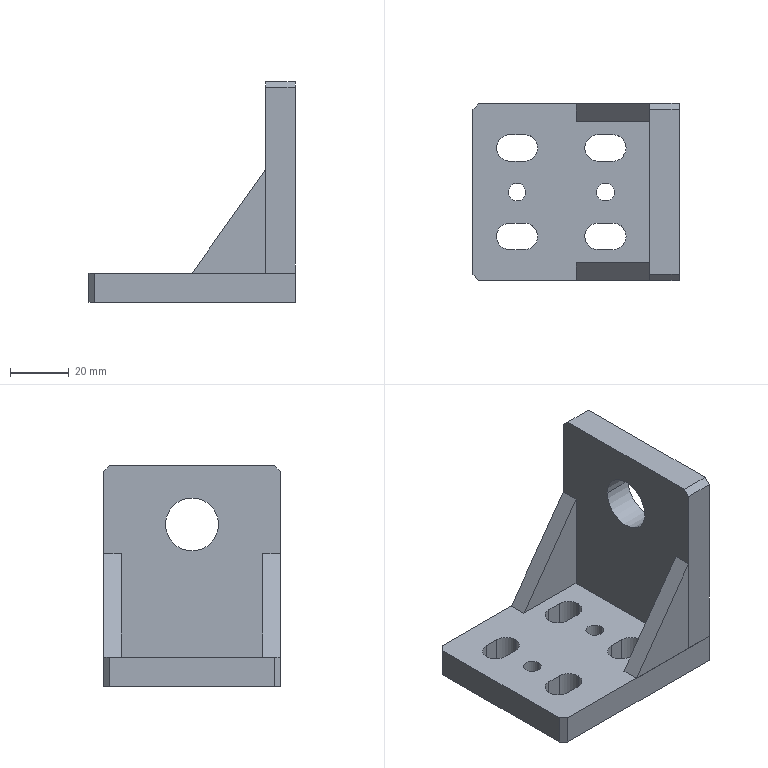Part | STEP file | Hydraulic Cylinder Connecting Bracket | 4 solids | 52 faces | box 70 x 60 x 75 mm | volume 78715 mm3 | plane 34 | cylinder 18 | commonest cylinder face diameters 9 x12 6 x4 18 x2
STEP:
#1=CARTESIAN_POINT('',(-13.,15.,0.));
#2=VERTEX_POINT('',#1);
#3=CARTESIAN_POINT('',(-17.5,19.5,0.));
#4=VERTEX_POINT('',#3);
#5=CARTESIAN_POINT('',(-17.5,15.,0.));
#6=DIRECTION('',(0.,0.,1.));
#7=DIRECTION('',(1.,0.,0.));
#8=AXIS2_PLACEMENT_3D('',#5,#6,#7);
#9=CIRCLE('',#8,4.5);
#10=EDGE_CURVE('',#2,#4,#9,.T.);
#11=ORIENTED_EDGE('',*,*,#10,.F.);
#12=CARTESIAN_POINT('',(-13.,15.,10.));
#13=VERTEX_POINT('',#12);
#14=CARTESIAN_POINT('',(-13.,15.,0.));
#15=DIRECTION('',(0.,0.,1.));
#16=VECTOR('',#15,1000.);
#17=LINE('',#14,#16);
#18=EDGE_CURVE('',#2,#13,#17,.T.);
#19=ORIENTED_EDGE('',*,*,#18,.T.);
#20=CARTESIAN_POINT('',(-17.5,19.5,10.));
#21=VERTEX_POINT('',#20);
#22=CARTESIAN_POINT('',(-17.5,15.,10.));
#23=DIRECTION('',(0.,0.,1.));
#24=DIRECTION('',(1.,0.,0.));
#25=AXIS2_PLACEMENT_3D('',#22,#23,#24);
#26=CIRCLE('',#25,4.5);
#27=EDGE_CURVE('',#13,#21,#26,.T.);
#28=ORIENTED_EDGE('',*,*,#27,.T.);
#29=CARTESIAN_POINT('',(-17.5,19.5,0.));
#30=DIRECTION('',(0.,0.,-1.));
#31=VECTOR('',#30,1000.);
#32=LINE('',#29,#31);
#33=EDGE_CURVE('',#21,#4,#32,.T.);
#34=ORIENTED_EDGE('',*,*,#33,.T.);
#35=EDGE_LOOP('',(#11,#19,#28,#34));
#36=FACE_OUTER_BOUND('',#35,.T.);
#37=CARTESIAN_POINT('',(-17.5,15.,0.));
#38=DIRECTION('',(0.,0.,1.));
#39=DIRECTION('',(1.,0.,0.));
#40=AXIS2_PLACEMENT_3D('',#37,#38,#39);
#41=CYLINDRICAL_SURFACE('',#40,4.5);
#42=ADVANCED_FACE('',(#36),#41,.F.);
#43=CARTESIAN_POINT('',(17.,15.,0.));
#44=VERTEX_POINT('',#43);
#45=CARTESIAN_POINT('',(12.5,19.5,0.));
#46=VERTEX_POINT('',#45);
#47=CARTESIAN_POINT('',(12.5,15.,0.));
#48=DIRECTION('',(0.,0.,1.));
#49=DIRECTION('',(1.,0.,0.));
#50=AXIS2_PLACEMENT_3D('',#47,#48,#49);
#51=CIRCLE('',#50,4.5);
#52=EDGE_CURVE('',#44,#46,#51,.T.);
#53=ORIENTED_EDGE('',*,*,#52,.F.);
#54=CARTESIAN_POINT('',(17.,15.,10.));
#55=VERTEX_POINT('',#54);
#56=CARTESIAN_POINT('',(17.,15.,0.));
#57=DIRECTION('',(0.,0.,1.));
#58=VECTOR('',#57,1000.);
#59=LINE('',#56,#58);
#60=EDGE_CURVE('',#44,#55,#59,.T.);
#61=ORIENTED_EDGE('',*,*,#60,.T.);
#62=CARTESIAN_POINT('',(12.5,19.5,10.));
#63=VERTEX_POINT('',#62);
#64=CARTESIAN_POINT('',(12.5,15.,10.));
#65=DIRECTION('',(0.,0.,1.));
#66=DIRECTION('',(1.,0.,0.));
#67=AXIS2_PLACEMENT_3D('',#64,#65,#66);
#68=CIRCLE('',#67,4.5);
#69=EDGE_CURVE('',#55,#63,#68,.T.);
#70=ORIENTED_EDGE('',*,*,#69,.T.);
#71=CARTESIAN_POINT('',(12.5,19.5,0.));
#72=DIRECTION('',(0.,0.,-1.));
#73=VECTOR('',#72,1000.);
#74=LINE('',#71,#73);
#75=EDGE_CURVE('',#63,#46,#74,.T.);
#76=ORIENTED_EDGE('',*,*,#75,.T.);
#77=EDGE_LOOP('',(#53,#61,#70,#76));
#78=FACE_OUTER_BOUND('',#77,.T.);
#79=CARTESIAN_POINT('',(12.5,15.,0.));
#80=DIRECTION('',(0.,0.,1.));
#81=DIRECTION('',(1.,0.,0.));
#82=AXIS2_PLACEMENT_3D('',#79,#80,#81);
#83=CYLINDRICAL_SURFACE('',#82,4.5);
#84=ADVANCED_FACE('',(#78),#83,.F.);
#85=CARTESIAN_POINT('',(17.,-15.,0.));
#86=VERTEX_POINT('',#85);
#87=CARTESIAN_POINT('',(12.5,-10.5,0.));
#88=VERTEX_POINT('',#87);
#89=CARTESIAN_POINT('',(12.5,-15.,0.));
#90=DIRECTION('',(0.,0.,1.));
#91=DIRECTION('',(1.,0.,0.));
#92=AXIS2_PLACEMENT_3D('',#89,#90,#91);
#93=CIRCLE('',#92,4.5);
#94=EDGE_CURVE('',#86,#88,#93,.T.);
#95=ORIENTED_EDGE('',*,*,#94,.F.);
#96=CARTESIAN_POINT('',(17.,-15.,10.));
#97=VERTEX_POINT('',#96);
#98=CARTESIAN_POINT('',(17.,-15.,0.));
#99=DIRECTION('',(0.,0.,1.));
#100=VECTOR('',#99,1000.);
#101=LINE('',#98,#100);
#102=EDGE_CURVE('',#86,#97,#101,.T.);
#103=ORIENTED_EDGE('',*,*,#102,.T.);
#104=CARTESIAN_POINT('',(12.5,-10.5,10.));
#105=VERTEX_POINT('',#104);
#106=CARTESIAN_POINT('',(12.5,-15.,10.));
#107=DIRECTION('',(0.,0.,1.));
#108=DIRECTION('',(1.,0.,0.));
#109=AXIS2_PLACEMENT_3D('',#106,#107,#108);
#110=CIRCLE('',#109,4.5);
#111=EDGE_CURVE('',#97,#105,#110,.T.);
#112=ORIENTED_EDGE('',*,*,#111,.T.);
#113=CARTESIAN_POINT('',(12.5,-10.5,0.));
#114=DIRECTION('',(0.,0.,-1.));
#115=VECTOR('',#114,1000.);
#116=LINE('',#113,#115);
#117=EDGE_CURVE('',#105,#88,#116,.T.);
#118=ORIENTED_EDGE('',*,*,#117,.T.);
#119=EDGE_LOOP('',(#95,#103,#112,#118));
#120=FACE_OUTER_BOUND('',#119,.T.);
#121=CARTESIAN_POINT('',(12.5,-15.,0.));
#122=DIRECTION('',(0.,0.,1.));
#123=DIRECTION('',(1.,0.,0.));
#124=AXIS2_PLACEMENT_3D('',#121,#122,#123);
#125=CYLINDRICAL_SURFACE('',#124,4.5);
#126=ADVANCED_FACE('',(#120),#125,.F.);
#127=CARTESIAN_POINT('',(-13.,-15.,0.));
#128=VERTEX_POINT('',#127);
#129=CARTESIAN_POINT('',(-17.5,-10.5,0.));
#130=VERTEX_POINT('',#129);
#131=CARTESIAN_POINT('',(-17.5,-15.,0.));
#132=DIRECTION('',(0.,0.,1.));
#133=DIRECTION('',(1.,0.,0.));
#134=AXIS2_PLACEMENT_3D('',#131,#132,#133);
#135=CIRCLE('',#134,4.5);
#136=EDGE_CURVE('',#128,#130,#135,.T.);
#137=ORIENTED_EDGE('',*,*,#136,.F.);
#138=CARTESIAN_POINT('',(-13.,-15.,10.));
#139=VERTEX_POINT('',#138);
#140=CARTESIAN_POINT('',(-13.,-15.,0.));
#141=DIRECTION('',(0.,0.,1.));
#142=VECTOR('',#141,1000.);
#143=LINE('',#140,#142);
#144=EDGE_CURVE('',#128,#139,#143,.T.);
#145=ORIENTED_EDGE('',*,*,#144,.T.);
#146=CARTESIAN_POINT('',(-17.5,-10.5,10.));
#147=VERTEX_POINT('',#146);
#148=CARTESIAN_POINT('',(-17.5,-15.,10.));
#149=DIRECTION('',(0.,0.,1.));
#150=DIRECTION('',(1.,0.,0.));
#151=AXIS2_PLACEMENT_3D('',#148,#149,#150);
#152=CIRCLE('',#151,4.5);
#153=EDGE_CURVE('',#139,#147,#152,.T.);
#154=ORIENTED_EDGE('',*,*,#153,.T.);
#155=CARTESIAN_POINT('',(-17.5,-10.5,0.));
#156=DIRECTION('',(0.,0.,-1.));
#157=VECTOR('',#156,1000.);
#158=LINE('',#155,#157);
#159=EDGE_CURVE('',#147,#130,#158,.T.);
#160=ORIENTED_EDGE('',*,*,#159,.T.);
#161=EDGE_LOOP('',(#137,#145,#154,#160));
#162=FACE_OUTER_BOUND('',#161,.T.);
#163=CARTESIAN_POINT('',(-17.5,-15.,0.));
#164=DIRECTION('',(0.,0.,1.));
#165=DIRECTION('',(1.,0.,0.));
#166=AXIS2_PLACEMENT_3D('',#163,#164,#165);
#167=CYLINDRICAL_SURFACE('',#166,4.5);
#168=ADVANCED_FACE('',(#162),#167,.F.);
#169=CARTESIAN_POINT('',(-23.,0.,0.));
#170=VERTEX_POINT('',#169);
#171=CARTESIAN_POINT('',(-17.,0.,0.));
#172=VERTEX_POINT('',#171);
#173=CARTESIAN_POINT('',(-20.,0.,0.));
#174=DIRECTION('',(0.,0.,1.));
#175=DIRECTION('',(1.,0.,0.));
#176=AXIS2_PLACEMENT_3D('',#173,#174,#175);
#177=CIRCLE('',#176,3.);
#178=EDGE_CURVE('',#170,#172,#177,.T.);
#179=ORIENTED_EDGE('',*,*,#178,.F.);
#180=CARTESIAN_POINT('',(-23.,0.,10.));
#181=VERTEX_POINT('',#180);
#182=CARTESIAN_POINT('',(-23.,0.,0.));
#183=DIRECTION('',(0.,0.,1.));
#184=VECTOR('',#183,1000.);
#185=LINE('',#182,#184);
#186=EDGE_CURVE('',#170,#181,#185,.T.);
#187=ORIENTED_EDGE('',*,*,#186,.T.);
#188=CARTESIAN_POINT('',(-17.,0.,10.));
#189=VERTEX_POINT('',#188);
#190=CARTESIAN_POINT('',(-20.,0.,10.));
#191=DIRECTION('',(0.,0.,1.));
#192=DIRECTION('',(1.,0.,0.));
#193=AXIS2_PLACEMENT_3D('',#190,#191,#192);
#194=CIRCLE('',#193,3.);
#195=EDGE_CURVE('',#181,#189,#194,.T.);
#196=ORIENTED_EDGE('',*,*,#195,.T.);
#197=CARTESIAN_POINT('',(-17.,0.,0.));
#198=DIRECTION('',(0.,0.,1.));
#199=VECTOR('',#198,1000.);
#200=LINE('',#197,#199);
#201=EDGE_CURVE('',#172,#189,#200,.T.);
#202=ORIENTED_EDGE('',*,*,#201,.F.);
#203=EDGE_LOOP('',(#179,#187,#196,#202));
#204=FACE_OUTER_BOUND('',#203,.T.);
#205=CARTESIAN_POINT('',(-20.,0.,0.));
#206=DIRECTION('',(0.,0.,1.));
#207=DIRECTION('',(1.,0.,0.));
#208=AXIS2_PLACEMENT_3D('',#205,#206,#207);
#209=CYLINDRICAL_SURFACE('',#208,3.);
#210=ADVANCED_FACE('',(#204),#209,.F.);
#211=CARTESIAN_POINT('',(7.,0.,0.));
#212=VERTEX_POINT('',#211);
#213=CARTESIAN_POINT('',(13.,0.,0.));
#214=VERTEX_POINT('',#213);
#215=CARTESIAN_POINT('',(10.,0.,0.));
#216=DIRECTION('',(0.,0.,1.));
#217=DIRECTION('',(1.,0.,0.));
#218=AXIS2_PLACEMENT_3D('',#215,#216,#217);
#219=CIRCLE('',#218,3.);
#220=EDGE_CURVE('',#212,#214,#219,.T.);
#221=ORIENTED_EDGE('',*,*,#220,.F.);
#222=CARTESIAN_POINT('',(7.,0.,10.));
#223=VERTEX_POINT('',#222);
#224=CARTESIAN_POINT('',(7.,0.,0.));
#225=DIRECTION('',(0.,0.,1.));
#226=VECTOR('',#225,1000.);
#227=LINE('',#224,#226);
#228=EDGE_CURVE('',#212,#223,#227,.T.);
#229=ORIENTED_EDGE('',*,*,#228,.T.);
#230=CARTESIAN_POINT('',(13.,0.,10.));
#231=VERTEX_POINT('',#230);
#232=CARTESIAN_POINT('',(10.,0.,10.));
#233=DIRECTION('',(0.,0.,1.));
#234=DIRECTION('',(1.,0.,0.));
#235=AXIS2_PLACEMENT_3D('',#232,#233,#234);
#236=CIRCLE('',#235,3.);
#237=EDGE_CURVE('',#223,#231,#236,.T.);
#238=ORIENTED_EDGE('',*,*,#237,.T.);
#239=CARTESIAN_POINT('',(13.,0.,0.));
#240=DIRECTION('',(0.,0.,1.));
#241=VECTOR('',#240,1000.);
#242=LINE('',#239,#241);
#243=EDGE_CURVE('',#214,#231,#242,.T.);
#244=ORIENTED_EDGE('',*,*,#243,.F.);
#245=EDGE_LOOP('',(#221,#229,#238,#244));
#246=FACE_OUTER_BOUND('',#245,.T.);
#247=CARTESIAN_POINT('',(10.,0.,0.));
#248=DIRECTION('',(0.,0.,1.));
#249=DIRECTION('',(1.,0.,0.));
#250=AXIS2_PLACEMENT_3D('',#247,#248,#249);
#251=CYLINDRICAL_SURFACE('',#250,3.);
#252=ADVANCED_FACE('',(#246),#251,.F.);
#253=CARTESIAN_POINT('',(-33.,-30.,10.));
#254=VERTEX_POINT('',#253);
#255=CARTESIAN_POINT('',(-35.,-28.,10.));
#256=VERTEX_POINT('',#255);
#257=CARTESIAN_POINT('',(-33.,-30.,10.));
#258=DIRECTION('',(-0.7071,0.7071,0.));
#259=VECTOR('',#258,1000.);
#260=LINE('',#257,#259);
#261=EDGE_CURVE('',#254,#256,#260,.T.);
#262=ORIENTED_EDGE('',*,*,#261,.F.);
#263=CARTESIAN_POINT('',(35.,-30.,10.));
#264=VERTEX_POINT('',#263);
#265=CARTESIAN_POINT('',(0.,-30.,10.));
#266=DIRECTION('',(-1.,0.,0.));
#267=VECTOR('',#266,1000.);
#268=LINE('',#265,#267);
#269=EDGE_CURVE('',#264,#254,#268,.T.);
#270=ORIENTED_EDGE('',*,*,#269,.F.);
#271=CARTESIAN_POINT('',(35.,30.,10.));
#272=VERTEX_POINT('',#271);
#273=CARTESIAN_POINT('',(35.,0.,10.));
#274=DIRECTION('',(0.,-1.,0.));
#275=VECTOR('',#274,1000.);
#276=LINE('',#273,#275);
#277=EDGE_CURVE('',#272,#264,#276,.T.);
#278=ORIENTED_EDGE('',*,*,#277,.F.);
#279=CARTESIAN_POINT('',(-33.,30.,10.));
#280=VERTEX_POINT('',#279);
#281=CARTESIAN_POINT('',(0.,30.,10.));
#282=DIRECTION('',(1.,0.,0.));
#283=VECTOR('',#282,1000.);
#284=LINE('',#281,#283);
#285=EDGE_CURVE('',#280,#272,#284,.T.);
#286=ORIENTED_EDGE('',*,*,#285,.F.);
#287=CARTESIAN_POINT('',(-35.,28.,10.));
#288=VERTEX_POINT('',#287);
#289=CARTESIAN_POINT('',(-35.,28.,10.));
#290=DIRECTION('',(0.7071,0.7071,0.));
#291=VECTOR('',#290,1000.);
#292=LINE('',#289,#291);
#293=EDGE_CURVE('',#288,#280,#292,.T.);
#294=ORIENTED_EDGE('',*,*,#293,.F.);
#295=CARTESIAN_POINT('',(-35.,0.,10.));
#296=DIRECTION('',(0.,1.,0.));
#297=VECTOR('',#296,1000.);
#298=LINE('',#295,#297);
#299=EDGE_CURVE('',#256,#288,#298,.T.);
#300=ORIENTED_EDGE('',*,*,#299,.F.);
#301=EDGE_LOOP('',(#262,#270,#278,#286,#294,#300));
#302=FACE_OUTER_BOUND('',#301,.T.);
#303=CARTESIAN_POINT('',(-22.5,19.5,10.));
#304=VERTEX_POINT('',#303);
#305=CARTESIAN_POINT('',(-22.5,10.5,10.));
#306=VERTEX_POINT('',#305);
#307=CARTESIAN_POINT('',(-22.5,15.,10.));
#308=DIRECTION('',(0.,0.,1.));
#309=DIRECTION('',(1.,0.,0.));
#310=AXIS2_PLACEMENT_3D('',#307,#308,#309);
#311=CIRCLE('',#310,4.5);
#312=EDGE_CURVE('',#304,#306,#311,.T.);
#313=ORIENTED_EDGE('',*,*,#312,.F.);
#314=CARTESIAN_POINT('',(0.,19.5,10.));
#315=DIRECTION('',(-1.,0.,0.));
#316=VECTOR('',#315,1000.);
#317=LINE('',#314,#316);
#318=EDGE_CURVE('',#21,#304,#317,.T.);
#319=ORIENTED_EDGE('',*,*,#318,.F.);
#320=ORIENTED_EDGE('',*,*,#27,.F.);
#321=CARTESIAN_POINT('',(-17.5,10.5,10.));
#322=VERTEX_POINT('',#321);
#323=CARTESIAN_POINT('',(-17.5,15.,10.));
#324=DIRECTION('',(0.,0.,1.));
#325=DIRECTION('',(1.,0.,0.));
#326=AXIS2_PLACEMENT_3D('',#323,#324,#325);
#327=CIRCLE('',#326,4.5);
#328=EDGE_CURVE('',#322,#13,#327,.T.);
#329=ORIENTED_EDGE('',*,*,#328,.F.);
#330=CARTESIAN_POINT('',(0.,10.5,10.));
#331=DIRECTION('',(1.,0.,0.));
#332=VECTOR('',#331,1000.);
#333=LINE('',#330,#332);
#334=EDGE_CURVE('',#306,#322,#333,.T.);
#335=ORIENTED_EDGE('',*,*,#334,.F.);
#336=EDGE_LOOP('',(#313,#319,#320,#329,#335));
#337=FACE_BOUND('',#336,.T.);
#338=CARTESIAN_POINT('',(7.5,19.5,10.));
#339=VERTEX_POINT('',#338);
#340=CARTESIAN_POINT('',(7.5,10.5,10.));
#341=VERTEX_POINT('',#340);
#342=CARTESIAN_POINT('',(7.5,15.,10.));
#343=DIRECTION('',(0.,0.,1.));
#344=DIRECTION('',(1.,0.,0.));
#345=AXIS2_PLACEMENT_3D('',#342,#343,#344);
#346=CIRCLE('',#345,4.5);
#347=EDGE_CURVE('',#339,#341,#346,.T.);
#348=ORIENTED_EDGE('',*,*,#347,.F.);
#349=CARTESIAN_POINT('',(0.,19.5,10.));
#350=DIRECTION('',(-1.,0.,0.));
#351=VECTOR('',#350,1000.);
#352=LINE('',#349,#351);
#353=EDGE_CURVE('',#63,#339,#352,.T.);
#354=ORIENTED_EDGE('',*,*,#353,.F.);
#355=ORIENTED_EDGE('',*,*,#69,.F.);
#356=CARTESIAN_POINT('',(12.5,10.5,10.));
#357=VERTEX_POINT('',#356);
#358=CARTESIAN_POINT('',(12.5,15.,10.));
#359=DIRECTION('',(0.,0.,1.));
#360=DIRECTION('',(1.,0.,0.));
#361=AXIS2_PLACEMENT_3D('',#358,#359,#360);
#362=CIRCLE('',#361,4.5);
#363=EDGE_CURVE('',#357,#55,#362,.T.);
#364=ORIENTED_EDGE('',*,*,#363,.F.);
#365=CARTESIAN_POINT('',(0.,10.5,10.));
#366=DIRECTION('',(1.,0.,0.));
#367=VECTOR('',#366,1000.);
#368=LINE('',#365,#367);
#369=EDGE_CURVE('',#341,#357,#368,.T.);
#370=ORIENTED_EDGE('',*,*,#369,.F.);
#371=EDGE_LOOP('',(#348,#354,#355,#364,#370));
#372=FACE_BOUND('',#371,.T.);
#373=CARTESIAN_POINT('',(7.5,-10.5,10.));
#374=VERTEX_POINT('',#373);
#375=CARTESIAN_POINT('',(7.5,-19.5,10.));
#376=VERTEX_POINT('',#375);
#377=CARTESIAN_POINT('',(7.5,-15.,10.));
#378=DIRECTION('',(0.,0.,1.));
#379=DIRECTION('',(1.,0.,0.));
#380=AXIS2_PLACEMENT_3D('',#377,#378,#379);
#381=CIRCLE('',#380,4.5);
#382=EDGE_CURVE('',#374,#376,#381,.T.);
#383=ORIENTED_EDGE('',*,*,#382,.F.);
#384=CARTESIAN_POINT('',(0.,-10.5,10.));
#385=DIRECTION('',(-1.,0.,0.));
#386=VECTOR('',#385,1000.);
#387=LINE('',#384,#386);
#388=EDGE_CURVE('',#105,#374,#387,.T.);
#389=ORIENTED_EDGE('',*,*,#388,.F.);
#390=ORIENTED_EDGE('',*,*,#111,.F.);
#391=CARTESIAN_POINT('',(12.5,-19.5,10.));
#392=VERTEX_POINT('',#391);
#393=CARTESIAN_POINT('',(12.5,-15.,10.));
#394=DIRECTION('',(0.,0.,1.));
#395=DIRECTION('',(1.,0.,0.));
#396=AXIS2_PLACEMENT_3D('',#393,#394,#395);
#397=CIRCLE('',#396,4.5);
#398=EDGE_CURVE('',#392,#97,#397,.T.);
#399=ORIENTED_EDGE('',*,*,#398,.F.);
#400=CARTESIAN_POINT('',(0.,-19.5,10.));
#401=DIRECTION('',(1.,0.,0.));
#402=VECTOR('',#401,1000.);
#403=LINE('',#400,#402);
#404=EDGE_CURVE('',#376,#392,#403,.T.);
#405=ORIENTED_EDGE('',*,*,#404,.F.);
#406=EDGE_LOOP('',(#383,#389,#390,#399,#405));
#407=FACE_BOUND('',#406,.T.);
#408=CARTESIAN_POINT('',(-22.5,-10.5,10.));
#409=VERTEX_POINT('',#408);
#410=CARTESIAN_POINT('',(-22.5,-19.5,10.));
#411=VERTEX_POINT('',#410);
#412=CARTESIAN_POINT('',(-22.5,-15.,10.));
#413=DIRECTION('',(0.,0.,1.));
#414=DIRECTION('',(1.,0.,0.));
#415=AXIS2_PLACEMENT_3D('',#412,#413,#414);
#416=CIRCLE('',#415,4.5);
#417=EDGE_CURVE('',#409,#411,#416,.T.);
#418=ORIENTED_EDGE('',*,*,#417,.F.);
#419=CARTESIAN_POINT('',(0.,-10.5,10.));
#420=DIRECTION('',(-1.,0.,0.));
#421=VECTOR('',#420,1000.);
#422=LINE('',#419,#421);
#423=EDGE_CURVE('',#147,#409,#422,.T.);
#424=ORIENTED_EDGE('',*,*,#423,.F.);
#425=ORIENTED_EDGE('',*,*,#153,.F.);
#426=CARTESIAN_POINT('',(-17.5,-19.5,10.));
#427=VERTEX_POINT('',#426);
#428=CARTESIAN_POINT('',(-17.5,-15.,10.));
#429=DIRECTION('',(0.,0.,1.));
#430=DIRECTION('',(1.,0.,0.));
#431=AXIS2_PLACEMENT_3D('',#428,#429,#430);
#432=CIRCLE('',#431,4.5);
#433=EDGE_CURVE('',#427,#139,#432,.T.);
#434=ORIENTED_EDGE('',*,*,#433,.F.);
#435=CARTESIAN_POINT('',(0.,-19.5,10.));
#436=DIRECTION('',(1.,0.,0.));
#437=VECTOR('',#436,1000.);
#438=LINE('',#435,#437);
#439=EDGE_CURVE('',#411,#427,#438,.T.);
#440=ORIENTED_EDGE('',*,*,#439,.F.);
#441=EDGE_LOOP('',(#418,#424,#425,#434,#440));
#442=FACE_BOUND('',#441,.T.);
#443=CARTESIAN_POINT('',(-20.,0.,10.));
#444=DIRECTION('',(0.,0.,1.));
#445=DIRECTION('',(1.,0.,0.));
#446=AXIS2_PLACEMENT_3D('',#443,#444,#445);
#447=CIRCLE('',#446,3.);
#448=EDGE_CURVE('',#189,#181,#447,.T.);
#449=ORIENTED_EDGE('',*,*,#448,.F.);
#450=ORIENTED_EDGE('',*,*,#195,.F.);
#451=EDGE_LOOP('',(#449,#450));
#452=FACE_BOUND('',#451,.T.);
#453=CARTESIAN_POINT('',(10.,0.,10.));
#454=DIRECTION('',(0.,0.,1.));
#455=DIRECTION('',(1.,0.,0.));
#456=AXIS2_PLACEMENT_3D('',#453,#454,#455);
#457=CIRCLE('',#456,3.);
#458=EDGE_CURVE('',#231,#223,#457,.T.);
#459=ORIENTED_EDGE('',*,*,#458,.F.);
#460=ORIENTED_EDGE('',*,*,#237,.F.);
#461=EDGE_LOOP('',(#459,#460));
#462=FACE_BOUND('',#461,.T.);
#463=CARTESIAN_POINT('',(0.,0.,10.));
#464=DIRECTION('',(0.,0.,-1.));
#465=DIRECTION('',(-1.,0.,0.));
#466=AXIS2_PLACEMENT_3D('',#463,#464,#465);
#467=PLANE('',#466);
#468=ADVANCED_FACE('',(#302,#337,#372,#407,#442,#452,#462),#467,.F.);
#469=ORIENTED_EDGE('',*,*,#299,.T.);
#470=CARTESIAN_POINT('',(-35.,28.,0.));
#471=VERTEX_POINT('',#470);
#472=CARTESIAN_POINT('',(-35.,28.,10.));
#473=DIRECTION('',(0.,0.,-1.));
#474=VECTOR('',#473,1000.);
#475=LINE('',#472,#474);
#476=EDGE_CURVE('',#288,#471,#475,.T.);
#477=ORIENTED_EDGE('',*,*,#476,.T.);
#478=CARTESIAN_POINT('',(-35.,-28.,0.));
#479=VERTEX_POINT('',#478);
#480=CARTESIAN_POINT('',(-35.,-30.,0.));
#481=DIRECTION('',(0.,-1.,0.));
#482=VECTOR('',#481,1000.);
#483=LINE('',#480,#482);
#484=EDGE_CURVE('',#471,#479,#483,.T.);
#485=ORIENTED_EDGE('',*,*,#484,.T.);
#486=CARTESIAN_POINT('',(-35.,-28.,10.));
#487=DIRECTION('',(0.,0.,1.));
#488=VECTOR('',#487,1000.);
#489=LINE('',#486,#488);
#490=EDGE_CURVE('',#479,#256,#489,.T.);
#491=ORIENTED_EDGE('',*,*,#490,.T.);
#492=EDGE_LOOP('',(#469,#477,#485,#491));
#493=FACE_OUTER_BOUND('',#492,.T.);
#494=CARTESIAN_POINT('',(-35.,-30.,10.));
#495=DIRECTION('',(-1.,0.,0.));
#496=DIRECTION('',(0.,0.,1.));
#497=AXIS2_PLACEMENT_3D('',#494,#495,#496);
#498=PLANE('',#497);
#499=ADVANCED_FACE('',(#493),#498,.T.);
#500=CARTESIAN_POINT('',(-33.,-30.,0.));
#501=VERTEX_POINT('',#500);
#502=CARTESIAN_POINT('',(-33.,-30.,0.));
#503=DIRECTION('',(0.7071,-0.7071,0.));
#504=VECTOR('',#503,1000.);
#505=LINE('',#502,#504);
#506=EDGE_CURVE('',#479,#501,#505,.T.);
#507=ORIENTED_EDGE('',*,*,#506,.T.);
#508=CARTESIAN_POINT('',(-33.,-30.,10.));
#509=DIRECTION('',(0.,0.,1.));
#510=VECTOR('',#509,1000.);
#511=LINE('',#508,#510);
#512=EDGE_CURVE('',#501,#254,#511,.T.);
#513=ORIENTED_EDGE('',*,*,#512,.T.);
#514=ORIENTED_EDGE('',*,*,#261,.T.);
#515=ORIENTED_EDGE('',*,*,#490,.F.);
#516=EDGE_LOOP('',(#507,#513,#514,#515));
#517=FACE_OUTER_BOUND('',#516,.T.);
#518=CARTESIAN_POINT('',(-33.,-30.,10.));
#519=DIRECTION('',(-0.7071,-0.7071,0.));
#520=DIRECTION('',(0.7071,-0.7071,0.));
#521=AXIS2_PLACEMENT_3D('',#518,#519,#520);
#522=PLANE('',#521);
#523=ADVANCED_FACE('',(#517),#522,.T.);
#524=ORIENTED_EDGE('',*,*,#512,.F.);
#525=CARTESIAN_POINT('',(35.,-30.,0.));
#526=VERTEX_POINT('',#525);
#527=CARTESIAN_POINT('',(-35.,-30.,0.));
#528=DIRECTION('',(-1.,0.,0.));
#529=VECTOR('',#528,1000.);
#530=LINE('',#527,#529);
#531=EDGE_CURVE('',#526,#501,#530,.T.);
#532=ORIENTED_EDGE('',*,*,#531,.F.);
#533=CARTESIAN_POINT('',(35.,-30.,10.));
#534=DIRECTION('',(0.,0.,-1.));
#535=VECTOR('',#534,1000.);
#536=LINE('',#533,#535);
#537=EDGE_CURVE('',#264,#526,#536,.T.);
#538=ORIENTED_EDGE('',*,*,#537,.F.);
#539=ORIENTED_EDGE('',*,*,#269,.T.);
#540=EDGE_LOOP('',(#524,#532,#538,#539));
#541=FACE_OUTER_BOUND('',#540,.T.);
#542=CARTESIAN_POINT('',(-35.,-30.,10.));
#543=DIRECTION('',(0.,1.,0.));
#544=DIRECTION('',(-1.,0.,0.));
#545=AXIS2_PLACEMENT_3D('',#542,#543,#544);
#546=PLANE('',#545);
#547=ADVANCED_FACE('',(#541),#546,.F.);
#548=ORIENTED_EDGE('',*,*,#277,.T.);
#549=ORIENTED_EDGE('',*,*,#537,.T.);
#550=CARTESIAN_POINT('',(35.,30.,0.));
#551=VERTEX_POINT('',#550);
#552=CARTESIAN_POINT('',(35.,30.,0.));
#553=DIRECTION('',(0.,1.,0.));
#554=VECTOR('',#553,1000.);
#555=LINE('',#552,#554);
#556=EDGE_CURVE('',#526,#551,#555,.T.);
#557=ORIENTED_EDGE('',*,*,#556,.T.);
#558=CARTESIAN_POINT('',(35.,30.,10.));
#559=DIRECTION('',(0.,0.,1.));
#560=VECTOR('',#559,1000.);
#561=LINE('',#558,#560);
#562=EDGE_CURVE('',#551,#272,#561,.T.);
#563=ORIENTED_EDGE('',*,*,#562,.T.);
#564=EDGE_LOOP('',(#548,#549,#557,#563));
#565=FACE_OUTER_BOUND('',#564,.T.);
#566=CARTESIAN_POINT('',(35.,30.,10.));
#567=DIRECTION('',(1.,0.,0.));
#568=DIRECTION('',(0.,0.,-1.));
#569=AXIS2_PLACEMENT_3D('',#566,#567,#568);
#570=PLANE('',#569);
#571=ADVANCED_FACE('',(#565),#570,.T.);
#572=ORIENTED_EDGE('',*,*,#285,.T.);
#573=ORIENTED_EDGE('',*,*,#562,.F.);
#574=CARTESIAN_POINT('',(-33.,30.,0.));
#575=VERTEX_POINT('',#574);
#576=CARTESIAN_POINT('',(-35.,30.,0.));
#577=DIRECTION('',(-1.,0.,0.));
#578=VECTOR('',#577,1000.);
#579=LINE('',#576,#578);
#580=EDGE_CURVE('',#551,#575,#579,.T.);
#581=ORIENTED_EDGE('',*,*,#580,.T.);
#582=CARTESIAN_POINT('',(-33.,30.,10.));
#583=DIRECTION('',(0.,0.,1.));
#584=VECTOR('',#583,1000.);
#585=LINE('',#582,#584);
#586=EDGE_CURVE('',#575,#280,#585,.T.);
#587=ORIENTED_EDGE('',*,*,#586,.T.);
#588=EDGE_LOOP('',(#572,#573,#581,#587));
#589=FACE_OUTER_BOUND('',#588,.T.);
#590=CARTESIAN_POINT('',(-35.,30.,10.));
#591=DIRECTION('',(0.,1.,0.));
#592=DIRECTION('',(-1.,0.,0.));
#593=AXIS2_PLACEMENT_3D('',#590,#591,#592);
#594=PLANE('',#593);
#595=ADVANCED_FACE('',(#589),#594,.T.);
#596=ORIENTED_EDGE('',*,*,#586,.F.);
#597=CARTESIAN_POINT('',(-35.,28.,0.));
#598=DIRECTION('',(0.7071,0.7071,0.));
#599=VECTOR('',#598,1000.);
#600=LINE('',#597,#599);
#601=EDGE_CURVE('',#471,#575,#600,.T.);
#602=ORIENTED_EDGE('',*,*,#601,.F.);
#603=ORIENTED_EDGE('',*,*,#476,.F.);
#604=ORIENTED_EDGE('',*,*,#293,.T.);
#605=EDGE_LOOP('',(#596,#602,#603,#604));
#606=FACE_OUTER_BOUND('',#605,.T.);
#607=CARTESIAN_POINT('',(-35.,28.,10.));
#608=DIRECTION('',(0.7071,-0.7071,0.));
#609=DIRECTION('',(0.7071,0.7071,0.));
#610=AXIS2_PLACEMENT_3D('',#607,#608,#609);
#611=PLANE('',#610);
#612=ADVANCED_FACE('',(#606),#611,.F.);
#613=CARTESIAN_POINT('',(-17.5,10.5,0.));
#614=VERTEX_POINT('',#613);
#615=CARTESIAN_POINT('',(-17.5,10.5,0.));
#616=DIRECTION('',(0.,0.,1.));
#617=VECTOR('',#616,1000.);
#618=LINE('',#615,#617);
#619=EDGE_CURVE('',#614,#322,#618,.T.);
#620=ORIENTED_EDGE('',*,*,#619,.F.);
#621=CARTESIAN_POINT('',(-22.5,10.5,0.));
#622=VERTEX_POINT('',#621);
#623=CARTESIAN_POINT('',(-22.5,10.5,0.));
#624=DIRECTION('',(1.,0.,0.));
#625=VECTOR('',#624,1000.);
#626=LINE('',#623,#625);
#627=EDGE_CURVE('',#622,#614,#626,.T.);
#628=ORIENTED_EDGE('',*,*,#627,.F.);
#629=CARTESIAN_POINT('',(-22.5,10.5,0.));
#630=DIRECTION('',(0.,0.,-1.));
#631=VECTOR('',#630,1000.);
#632=LINE('',#629,#631);
#633=EDGE_CURVE('',#306,#622,#632,.T.);
#634=ORIENTED_EDGE('',*,*,#633,.F.);
#635=ORIENTED_EDGE('',*,*,#334,.T.);
#636=EDGE_LOOP('',(#620,#628,#634,#635));
#637=FACE_OUTER_BOUND('',#636,.T.);
#638=CARTESIAN_POINT('',(-22.5,10.5,0.));
#639=DIRECTION('',(0.,-1.,0.));
#640=DIRECTION('',(1.,0.,0.));
#641=AXIS2_PLACEMENT_3D('',#638,#639,#640);
#642=PLANE('',#641);
#643=ADVANCED_FACE('',(#637),#642,.F.);
#644=ORIENTED_EDGE('',*,*,#633,.T.);
#645=CARTESIAN_POINT('',(-22.5,19.5,0.));
#646=VERTEX_POINT('',#645);
#647=CARTESIAN_POINT('',(-22.5,15.,0.));
#648=DIRECTION('',(0.,0.,1.));
#649=DIRECTION('',(1.,0.,0.));
#650=AXIS2_PLACEMENT_3D('',#647,#648,#649);
#651=CIRCLE('',#650,4.5);
#652=EDGE_CURVE('',#646,#622,#651,.T.);
#653=ORIENTED_EDGE('',*,*,#652,.F.);
#654=CARTESIAN_POINT('',(-22.5,19.5,0.));
#655=DIRECTION('',(0.,0.,-1.));
#656=VECTOR('',#655,1000.);
#657=LINE('',#654,#656);
#658=EDGE_CURVE('',#304,#646,#657,.T.);
#659=ORIENTED_EDGE('',*,*,#658,.F.);
#660=ORIENTED_EDGE('',*,*,#312,.T.);
#661=EDGE_LOOP('',(#644,#653,#659,#660));
#662=FACE_OUTER_BOUND('',#661,.T.);
#663=CARTESIAN_POINT('',(-22.5,15.,0.));
#664=DIRECTION('',(0.,0.,1.));
#665=DIRECTION('',(1.,0.,0.));
#666=AXIS2_PLACEMENT_3D('',#663,#664,#665);
#667=CYLINDRICAL_SURFACE('',#666,4.5);
#668=ADVANCED_FACE('',(#662),#667,.F.);
#669=ORIENTED_EDGE('',*,*,#658,.T.);
#670=CARTESIAN_POINT('',(-22.5,19.5,0.));
#671=DIRECTION('',(-1.,0.,0.));
#672=VECTOR('',#671,1000.);
#673=LINE('',#670,#672);
#674=EDGE_CURVE('',#4,#646,#673,.T.);
#675=ORIENTED_EDGE('',*,*,#674,.F.);
#676=ORIENTED_EDGE('',*,*,#33,.F.);
#677=ORIENTED_EDGE('',*,*,#318,.T.);
#678=EDGE_LOOP('',(#669,#675,#676,#677));
#679=FACE_OUTER_BOUND('',#678,.T.);
#680=CARTESIAN_POINT('',(-22.5,19.5,0.));
#681=DIRECTION('',(0.,1.,0.));
#682=DIRECTION('',(0.,0.,1.));
#683=AXIS2_PLACEMENT_3D('',#680,#681,#682);
#684=PLANE('',#683);
#685=ADVANCED_FACE('',(#679),#684,.F.);
#686=ORIENTED_EDGE('',*,*,#18,.F.);
#687=CARTESIAN_POINT('',(-17.5,15.,0.));
#688=DIRECTION('',(0.,0.,1.));
#689=DIRECTION('',(1.,0.,0.));
#690=AXIS2_PLACEMENT_3D('',#687,#688,#689);
#691=CIRCLE('',#690,4.5);
#692=EDGE_CURVE('',#614,#2,#691,.T.);
#693=ORIENTED_EDGE('',*,*,#692,.F.);
#694=ORIENTED_EDGE('',*,*,#619,.T.);
#695=ORIENTED_EDGE('',*,*,#328,.T.);
#696=EDGE_LOOP('',(#686,#693,#694,#695));
#697=FACE_OUTER_BOUND('',#696,.T.);
#698=CARTESIAN_POINT('',(-17.5,15.,0.));
#699=DIRECTION('',(0.,0.,1.));
#700=DIRECTION('',(1.,0.,0.));
#701=AXIS2_PLACEMENT_3D('',#698,#699,#700);
#702=CYLINDRICAL_SURFACE('',#701,4.5);
#703=ADVANCED_FACE('',(#697),#702,.F.);
#704=CARTESIAN_POINT('',(12.5,10.5,0.));
#705=VERTEX_POINT('',#704);
#706=CARTESIAN_POINT('',(12.5,10.5,0.));
#707=DIRECTION('',(0.,0.,1.));
#708=VECTOR('',#707,1000.);
#709=LINE('',#706,#708);
#710=EDGE_CURVE('',#705,#357,#709,.T.);
#711=ORIENTED_EDGE('',*,*,#710,.F.);
#712=CARTESIAN_POINT('',(7.5,10.5,0.));
#713=VERTEX_POINT('',#712);
#714=CARTESIAN_POINT('',(7.5,10.5,0.));
#715=DIRECTION('',(1.,0.,0.));
#716=VECTOR('',#715,1000.);
#717=LINE('',#714,#716);
#718=EDGE_CURVE('',#713,#705,#717,.T.);
#719=ORIENTED_EDGE('',*,*,#718,.F.);
#720=CARTESIAN_POINT('',(7.5,10.5,0.));
#721=DIRECTION('',(0.,0.,-1.));
#722=VECTOR('',#721,1000.);
#723=LINE('',#720,#722);
#724=EDGE_CURVE('',#341,#713,#723,.T.);
#725=ORIENTED_EDGE('',*,*,#724,.F.);
#726=ORIENTED_EDGE('',*,*,#369,.T.);
#727=EDGE_LOOP('',(#711,#719,#725,#726));
#728=FACE_OUTER_BOUND('',#727,.T.);
#729=CARTESIAN_POINT('',(7.5,10.5,0.));
#730=DIRECTION('',(0.,-1.,0.));
#731=DIRECTION('',(1.,0.,0.));
#732=AXIS2_PLACEMENT_3D('',#729,#730,#731);
#733=PLANE('',#732);
#734=ADVANCED_FACE('',(#728),#733,.F.);
#735=ORIENTED_EDGE('',*,*,#724,.T.);
#736=CARTESIAN_POINT('',(7.5,19.5,0.));
#737=VERTEX_POINT('',#736);
#738=CARTESIAN_POINT('',(7.5,15.,0.));
#739=DIRECTION('',(0.,0.,1.));
#740=DIRECTION('',(1.,0.,0.));
#741=AXIS2_PLACEMENT_3D('',#738,#739,#740);
#742=CIRCLE('',#741,4.5);
#743=EDGE_CURVE('',#737,#713,#742,.T.);
#744=ORIENTED_EDGE('',*,*,#743,.F.);
#745=CARTESIAN_POINT('',(7.5,19.5,0.));
#746=DIRECTION('',(0.,0.,-1.));
#747=VECTOR('',#746,1000.);
#748=LINE('',#745,#747);
#749=EDGE_CURVE('',#339,#737,#748,.T.);
#750=ORIENTED_EDGE('',*,*,#749,.F.);
#751=ORIENTED_EDGE('',*,*,#347,.T.);
#752=EDGE_LOOP('',(#735,#744,#750,#751));
#753=FACE_OUTER_BOUND('',#752,.T.);
#754=CARTESIAN_POINT('',(7.5,15.,0.));
#755=DIRECTION('',(0.,0.,1.));
#756=DIRECTION('',(1.,0.,0.));
#757=AXIS2_PLACEMENT_3D('',#754,#755,#756);
#758=CYLINDRICAL_SURFACE('',#757,4.5);
#759=ADVANCED_FACE('',(#753),#758,.F.);
#760=ORIENTED_EDGE('',*,*,#749,.T.);
#761=CARTESIAN_POINT('',(7.5,19.5,0.));
#762=DIRECTION('',(-1.,0.,0.));
#763=VECTOR('',#762,1000.);
#764=LINE('',#761,#763);
#765=EDGE_CURVE('',#46,#737,#764,.T.);
#766=ORIENTED_EDGE('',*,*,#765,.F.);
#767=ORIENTED_EDGE('',*,*,#75,.F.);
#768=ORIENTED_EDGE('',*,*,#353,.T.);
#769=EDGE_LOOP('',(#760,#766,#767,#768));
#770=FACE_OUTER_BOUND('',#769,.T.);
#771=CARTESIAN_POINT('',(7.5,19.5,0.));
#772=DIRECTION('',(0.,1.,0.));
#773=DIRECTION('',(0.,0.,1.));
#774=AXIS2_PLACEMENT_3D('',#771,#772,#773);
#775=PLANE('',#774);
#776=ADVANCED_FACE('',(#770),#775,.F.);
#777=ORIENTED_EDGE('',*,*,#60,.F.);
#778=CARTESIAN_POINT('',(12.5,15.,0.));
#779=DIRECTION('',(0.,0.,1.));
#780=DIRECTION('',(1.,0.,0.));
#781=AXIS2_PLACEMENT_3D('',#778,#779,#780);
#782=CIRCLE('',#781,4.5);
#783=EDGE_CURVE('',#705,#44,#782,.T.);
#784=ORIENTED_EDGE('',*,*,#783,.F.);
#785=ORIENTED_EDGE('',*,*,#710,.T.);
#786=ORIENTED_EDGE('',*,*,#363,.T.);
#787=EDGE_LOOP('',(#777,#784,#785,#786));
#788=FACE_OUTER_BOUND('',#787,.T.);
#789=CARTESIAN_POINT('',(12.5,15.,0.));
#790=DIRECTION('',(0.,0.,1.));
#791=DIRECTION('',(1.,0.,0.));
#792=AXIS2_PLACEMENT_3D('',#789,#790,#791);
#793=CYLINDRICAL_SURFACE('',#792,4.5);
#794=ADVANCED_FACE('',(#788),#793,.F.);
#795=CARTESIAN_POINT('',(12.5,-19.5,0.));
#796=VERTEX_POINT('',#795);
#797=CARTESIAN_POINT('',(12.5,-19.5,0.));
#798=DIRECTION('',(0.,0.,1.));
#799=VECTOR('',#798,1000.);
#800=LINE('',#797,#799);
#801=EDGE_CURVE('',#796,#392,#800,.T.);
#802=ORIENTED_EDGE('',*,*,#801,.F.);
#803=CARTESIAN_POINT('',(7.5,-19.5,0.));
#804=VERTEX_POINT('',#803);
#805=CARTESIAN_POINT('',(7.5,-19.5,0.));
#806=DIRECTION('',(1.,0.,0.));
#807=VECTOR('',#806,1000.);
#808=LINE('',#805,#807);
#809=EDGE_CURVE('',#804,#796,#808,.T.);
#810=ORIENTED_EDGE('',*,*,#809,.F.);
#811=CARTESIAN_POINT('',(7.5,-19.5,0.));
#812=DIRECTION('',(0.,0.,-1.));
#813=VECTOR('',#812,1000.);
#814=LINE('',#811,#813);
#815=EDGE_CURVE('',#376,#804,#814,.T.);
#816=ORIENTED_EDGE('',*,*,#815,.F.);
#817=ORIENTED_EDGE('',*,*,#404,.T.);
#818=EDGE_LOOP('',(#802,#810,#816,#817));
#819=FACE_OUTER_BOUND('',#818,.T.);
#820=CARTESIAN_POINT('',(7.5,-19.5,0.));
#821=DIRECTION('',(0.,-1.,0.));
#822=DIRECTION('',(0.,0.,-1.));
#823=AXIS2_PLACEMENT_3D('',#820,#821,#822);
#824=PLANE('',#823);
#825=ADVANCED_FACE('',(#819),#824,.F.);
#826=ORIENTED_EDGE('',*,*,#815,.T.);
#827=CARTESIAN_POINT('',(7.5,-10.5,0.));
#828=VERTEX_POINT('',#827);
#829=CARTESIAN_POINT('',(7.5,-15.,0.));
#830=DIRECTION('',(0.,0.,1.));
#831=DIRECTION('',(1.,0.,0.));
#832=AXIS2_PLACEMENT_3D('',#829,#830,#831);
#833=CIRCLE('',#832,4.5);
#834=EDGE_CURVE('',#828,#804,#833,.T.);
#835=ORIENTED_EDGE('',*,*,#834,.F.);
#836=CARTESIAN_POINT('',(7.5,-10.5,0.));
#837=DIRECTION('',(0.,0.,-1.));
#838=VECTOR('',#837,1000.);
#839=LINE('',#836,#838);
#840=EDGE_CURVE('',#374,#828,#839,.T.);
#841=ORIENTED_EDGE('',*,*,#840,.F.);
#842=ORIENTED_EDGE('',*,*,#382,.T.);
#843=EDGE_LOOP('',(#826,#835,#841,#842));
#844=FACE_OUTER_BOUND('',#843,.T.);
#845=CARTESIAN_POINT('',(7.5,-15.,0.));
#846=DIRECTION('',(0.,0.,1.));
#847=DIRECTION('',(1.,0.,0.));
#848=AXIS2_PLACEMENT_3D('',#845,#846,#847);
#849=CYLINDRICAL_SURFACE('',#848,4.5);
#850=ADVANCED_FACE('',(#844),#849,.F.);
#851=ORIENTED_EDGE('',*,*,#840,.T.);
#852=CARTESIAN_POINT('',(7.5,-10.5,0.));
#853=DIRECTION('',(-1.,0.,0.));
#854=VECTOR('',#853,1000.);
#855=LINE('',#852,#854);
#856=EDGE_CURVE('',#88,#828,#855,.T.);
#857=ORIENTED_EDGE('',*,*,#856,.F.);
#858=ORIENTED_EDGE('',*,*,#117,.F.);
#859=ORIENTED_EDGE('',*,*,#388,.T.);
#860=EDGE_LOOP('',(#851,#857,#858,#859));
#861=FACE_OUTER_BOUND('',#860,.T.);
#862=CARTESIAN_POINT('',(7.5,-10.5,0.));
#863=DIRECTION('',(0.,1.,0.));
#864=DIRECTION('',(-1.,0.,0.));
#865=AXIS2_PLACEMENT_3D('',#862,#863,#864);
#866=PLANE('',#865);
#867=ADVANCED_FACE('',(#861),#866,.F.);
#868=ORIENTED_EDGE('',*,*,#102,.F.);
#869=CARTESIAN_POINT('',(12.5,-15.,0.));
#870=DIRECTION('',(0.,0.,1.));
#871=DIRECTION('',(1.,0.,0.));
#872=AXIS2_PLACEMENT_3D('',#869,#870,#871);
#873=CIRCLE('',#872,4.5);
#874=EDGE_CURVE('',#796,#86,#873,.T.);
#875=ORIENTED_EDGE('',*,*,#874,.F.);
#876=ORIENTED_EDGE('',*,*,#801,.T.);
#877=ORIENTED_EDGE('',*,*,#398,.T.);
#878=EDGE_LOOP('',(#868,#875,#876,#877));
#879=FACE_OUTER_BOUND('',#878,.T.);
#880=CARTESIAN_POINT('',(12.5,-15.,0.));
#881=DIRECTION('',(0.,0.,1.));
#882=DIRECTION('',(1.,0.,0.));
#883=AXIS2_PLACEMENT_3D('',#880,#881,#882);
#884=CYLINDRICAL_SURFACE('',#883,4.5);
#885=ADVANCED_FACE('',(#879),#884,.F.);
#886=CARTESIAN_POINT('',(-17.5,-19.5,0.));
#887=VERTEX_POINT('',#886);
#888=CARTESIAN_POINT('',(-17.5,-19.5,0.));
#889=DIRECTION('',(0.,0.,1.));
#890=VECTOR('',#889,1000.);
#891=LINE('',#888,#890);
#892=EDGE_CURVE('',#887,#427,#891,.T.);
#893=ORIENTED_EDGE('',*,*,#892,.F.);
#894=CARTESIAN_POINT('',(-22.5,-19.5,0.));
#895=VERTEX_POINT('',#894);
#896=CARTESIAN_POINT('',(-22.5,-19.5,0.));
#897=DIRECTION('',(1.,0.,0.));
#898=VECTOR('',#897,1000.);
#899=LINE('',#896,#898);
#900=EDGE_CURVE('',#895,#887,#899,.T.);
#901=ORIENTED_EDGE('',*,*,#900,.F.);
#902=CARTESIAN_POINT('',(-22.5,-19.5,0.));
#903=DIRECTION('',(0.,0.,-1.));
#904=VECTOR('',#903,1000.);
#905=LINE('',#902,#904);
#906=EDGE_CURVE('',#411,#895,#905,.T.);
#907=ORIENTED_EDGE('',*,*,#906,.F.);
#908=ORIENTED_EDGE('',*,*,#439,.T.);
#909=EDGE_LOOP('',(#893,#901,#907,#908));
#910=FACE_OUTER_BOUND('',#909,.T.);
#911=CARTESIAN_POINT('',(-22.5,-19.5,0.));
#912=DIRECTION('',(0.,-1.,0.));
#913=DIRECTION('',(0.,0.,-1.));
#914=AXIS2_PLACEMENT_3D('',#911,#912,#913);
#915=PLANE('',#914);
#916=ADVANCED_FACE('',(#910),#915,.F.);
#917=ORIENTED_EDGE('',*,*,#906,.T.);
#918=CARTESIAN_POINT('',(-22.5,-10.5,0.));
#919=VERTEX_POINT('',#918);
#920=CARTESIAN_POINT('',(-22.5,-15.,0.));
#921=DIRECTION('',(0.,0.,1.));
#922=DIRECTION('',(1.,0.,0.));
#923=AXIS2_PLACEMENT_3D('',#920,#921,#922);
#924=CIRCLE('',#923,4.5);
#925=EDGE_CURVE('',#919,#895,#924,.T.);
#926=ORIENTED_EDGE('',*,*,#925,.F.);
#927=CARTESIAN_POINT('',(-22.5,-10.5,0.));
#928=DIRECTION('',(0.,0.,-1.));
#929=VECTOR('',#928,1000.);
#930=LINE('',#927,#929);
#931=EDGE_CURVE('',#409,#919,#930,.T.);
#932=ORIENTED_EDGE('',*,*,#931,.F.);
#933=ORIENTED_EDGE('',*,*,#417,.T.);
#934=EDGE_LOOP('',(#917,#926,#932,#933));
#935=FACE_OUTER_BOUND('',#934,.T.);
#936=CARTESIAN_POINT('',(-22.5,-15.,0.));
#937=DIRECTION('',(0.,0.,1.));
#938=DIRECTION('',(1.,0.,0.));
#939=AXIS2_PLACEMENT_3D('',#936,#937,#938);
#940=CYLINDRICAL_SURFACE('',#939,4.5);
#941=ADVANCED_FACE('',(#935),#940,.F.);
#942=ORIENTED_EDGE('',*,*,#931,.T.);
#943=CARTESIAN_POINT('',(-22.5,-10.5,0.));
#944=DIRECTION('',(-1.,0.,0.));
#945=VECTOR('',#944,1000.);
#946=LINE('',#943,#945);
#947=EDGE_CURVE('',#130,#919,#946,.T.);
#948=ORIENTED_EDGE('',*,*,#947,.F.);
#949=ORIENTED_EDGE('',*,*,#159,.F.);
#950=ORIENTED_EDGE('',*,*,#423,.T.);
#951=EDGE_LOOP('',(#942,#948,#949,#950));
#952=FACE_OUTER_BOUND('',#951,.T.);
#953=CARTESIAN_POINT('',(-22.5,-10.5,0.));
#954=DIRECTION('',(0.,1.,0.));
#955=DIRECTION('',(-1.,0.,0.));
#956=AXIS2_PLACEMENT_3D('',#953,#954,#955);
#957=PLANE('',#956);
#958=ADVANCED_FACE('',(#952),#957,.F.);
#959=ORIENTED_EDGE('',*,*,#144,.F.);
#960=CARTESIAN_POINT('',(-17.5,-15.,0.));
#961=DIRECTION('',(0.,0.,1.));
#962=DIRECTION('',(1.,0.,0.));
#963=AXIS2_PLACEMENT_3D('',#960,#961,#962);
#964=CIRCLE('',#963,4.5);
#965=EDGE_CURVE('',#887,#128,#964,.T.);
#966=ORIENTED_EDGE('',*,*,#965,.F.);
#967=ORIENTED_EDGE('',*,*,#892,.T.);
#968=ORIENTED_EDGE('',*,*,#433,.T.);
#969=EDGE_LOOP('',(#959,#966,#967,#968));
#970=FACE_OUTER_BOUND('',#969,.T.);
#971=CARTESIAN_POINT('',(-17.5,-15.,0.));
#972=DIRECTION('',(0.,0.,1.));
#973=DIRECTION('',(1.,0.,0.));
#974=AXIS2_PLACEMENT_3D('',#971,#972,#973);
#975=CYLINDRICAL_SURFACE('',#974,4.5);
#976=ADVANCED_FACE('',(#970),#975,.F.);
#977=ORIENTED_EDGE('',*,*,#186,.F.);
#978=CARTESIAN_POINT('',(-20.,0.,0.));
#979=DIRECTION('',(0.,0.,1.));
#980=DIRECTION('',(1.,0.,0.));
#981=AXIS2_PLACEMENT_3D('',#978,#979,#980);
#982=CIRCLE('',#981,3.);
#983=EDGE_CURVE('',#172,#170,#982,.T.);
#984=ORIENTED_EDGE('',*,*,#983,.F.);
#985=ORIENTED_EDGE('',*,*,#201,.T.);
#986=ORIENTED_EDGE('',*,*,#448,.T.);
#987=EDGE_LOOP('',(#977,#984,#985,#986));
#988=FACE_OUTER_BOUND('',#987,.T.);
#989=CARTESIAN_POINT('',(-20.,0.,0.));
#990=DIRECTION('',(0.,0.,1.));
#991=DIRECTION('',(1.,0.,0.));
#992=AXIS2_PLACEMENT_3D('',#989,#990,#991);
#993=CYLINDRICAL_SURFACE('',#992,3.);
#994=ADVANCED_FACE('',(#988),#993,.F.);
#995=ORIENTED_EDGE('',*,*,#228,.F.);
#996=CARTESIAN_POINT('',(10.,0.,0.));
#997=DIRECTION('',(0.,0.,1.));
#998=DIRECTION('',(1.,0.,0.));
#999=AXIS2_PLACEMENT_3D('',#996,#997,#998);
#1000=CIRCLE('',#999,3.);
#1001=EDGE_CURVE('',#214,#212,#1000,.T.);
#1002=ORIENTED_EDGE('',*,*,#1001,.F.);
#1003=ORIENTED_EDGE('',*,*,#243,.T.);
#1004=ORIENTED_EDGE('',*,*,#458,.T.);
#1005=EDGE_LOOP('',(#995,#1002,#1003,#1004));
#1006=FACE_OUTER_BOUND('',#1005,.T.);
#1007=CARTESIAN_POINT('',(10.,0.,0.));
#1008=DIRECTION('',(0.,0.,1.));
#1009=DIRECTION('',(1.,0.,0.));
#1010=AXIS2_PLACEMENT_3D('',#1007,#1008,#1009);
#1011=CYLINDRICAL_SURFACE('',#1010,3.);
#1012=ADVANCED_FACE('',(#1006),#1011,.F.);
#1013=ORIENTED_EDGE('',*,*,#580,.F.);
#1014=ORIENTED_EDGE('',*,*,#556,.F.);
#1015=ORIENTED_EDGE('',*,*,#531,.T.);
#1016=ORIENTED_EDGE('',*,*,#506,.F.);
#1017=ORIENTED_EDGE('',*,*,#484,.F.);
#1018=ORIENTED_EDGE('',*,*,#601,.T.);
#1019=EDGE_LOOP('',(#1013,#1014,#1015,#1016,#1017,#1018));
#1020=FACE_OUTER_BOUND('',#1019,.T.);
#1021=ORIENTED_EDGE('',*,*,#692,.T.);
#1022=ORIENTED_EDGE('',*,*,#10,.T.);
#1023=ORIENTED_EDGE('',*,*,#674,.T.);
#1024=ORIENTED_EDGE('',*,*,#652,.T.);
#1025=ORIENTED_EDGE('',*,*,#627,.T.);
#1026=EDGE_LOOP('',(#1021,#1022,#1023,#1024,#1025));
#1027=FACE_BOUND('',#1026,.T.);
#1028=ORIENTED_EDGE('',*,*,#783,.T.);
#1029=ORIENTED_EDGE('',*,*,#52,.T.);
#1030=ORIENTED_EDGE('',*,*,#765,.T.);
#1031=ORIENTED_EDGE('',*,*,#743,.T.);
#1032=ORIENTED_EDGE('',*,*,#718,.T.);
#1033=EDGE_LOOP('',(#1028,#1029,#1030,#1031,#1032));
#1034=FACE_BOUND('',#1033,.T.);
#1035=ORIENTED_EDGE('',*,*,#874,.T.);
#1036=ORIENTED_EDGE('',*,*,#94,.T.);
#1037=ORIENTED_EDGE('',*,*,#856,.T.);
#1038=ORIENTED_EDGE('',*,*,#834,.T.);
#1039=ORIENTED_EDGE('',*,*,#809,.T.);
#1040=EDGE_LOOP('',(#1035,#1036,#1037,#1038,#1039));
#1041=FACE_BOUND('',#1040,.T.);
#1042=ORIENTED_EDGE('',*,*,#965,.T.);
#1043=ORIENTED_EDGE('',*,*,#136,.T.);
#1044=ORIENTED_EDGE('',*,*,#947,.T.);
#1045=ORIENTED_EDGE('',*,*,#925,.T.);
#1046=ORIENTED_EDGE('',*,*,#900,.T.);
#1047=EDGE_LOOP('',(#1042,#1043,#1044,#1045,#1046));
#1048=FACE_BOUND('',#1047,.T.);
#1049=ORIENTED_EDGE('',*,*,#983,.T.);
#1050=ORIENTED_EDGE('',*,*,#178,.T.);
#1051=EDGE_LOOP('',(#1049,#1050));
#1052=FACE_BOUND('',#1051,.T.);
#1053=ORIENTED_EDGE('',*,*,#1001,.T.);
#1054=ORIENTED_EDGE('',*,*,#220,.T.);
#1055=EDGE_LOOP('',(#1053,#1054));
#1056=FACE_BOUND('',#1055,.T.);
#1057=CARTESIAN_POINT('',(0.,0.,0.));
#1058=DIRECTION('',(0.,0.,-1.));
#1059=DIRECTION('',(-1.,0.,0.));
#1060=AXIS2_PLACEMENT_3D('',#1057,#1058,#1059);
#1061=PLANE('',#1060);
#1062=ADVANCED_FACE('',(#1020,#1027,#1034,#1041,#1048,#1052,#1056),#1061,.T.);
#1063=CLOSED_SHELL('',(#42,#84,#126,#168,#210,#252,#468,#499,#523,#547,#571,#595,#612,#643,#668,#685,#703,#734,#759,#776,#794,#825,#850,#867,#885,#916,#941,#958,#976,#994,#1012,#1062));
#1064=MANIFOLD_SOLID_BREP('',#1063);
#1065=CARTESIAN_POINT('',(0.,24.,10.));
#1066=VERTEX_POINT('',#1065);
#1067=CARTESIAN_POINT('',(25.,24.,45.));
#1068=VERTEX_POINT('',#1067);
#1069=CARTESIAN_POINT('',(0.,24.,10.));
#1070=DIRECTION('',(0.5812,0.,0.8137));
#1071=VECTOR('',#1070,1000.);
#1072=LINE('',#1069,#1071);
#1073=EDGE_CURVE('',#1066,#1068,#1072,.T.);
#1074=ORIENTED_EDGE('',*,*,#1073,.F.);
#1075=CARTESIAN_POINT('',(25.,24.,10.));
#1076=VERTEX_POINT('',#1075);
#1077=CARTESIAN_POINT('',(0.,24.,10.));
#1078=DIRECTION('',(-1.,0.,0.));
#1079=VECTOR('',#1078,1000.);
#1080=LINE('',#1077,#1079);
#1081=EDGE_CURVE('',#1076,#1066,#1080,.T.);
#1082=ORIENTED_EDGE('',*,*,#1081,.F.);
#1083=CARTESIAN_POINT('',(25.,24.,0.));
#1084=DIRECTION('',(0.,0.,-1.));
#1085=VECTOR('',#1084,1000.);
#1086=LINE('',#1083,#1085);
#1087=EDGE_CURVE('',#1068,#1076,#1086,.T.);
#1088=ORIENTED_EDGE('',*,*,#1087,.F.);
#1089=EDGE_LOOP('',(#1074,#1082,#1088));
#1090=FACE_OUTER_BOUND('',#1089,.T.);
#1091=CARTESIAN_POINT('',(0.,24.,0.));
#1092=DIRECTION('',(0.,1.,0.));
#1093=DIRECTION('',(0.,0.,1.));
#1094=AXIS2_PLACEMENT_3D('',#1091,#1092,#1093);
#1095=PLANE('',#1094);
#1096=ADVANCED_FACE('',(#1090),#1095,.F.);
#1097=ORIENTED_EDGE('',*,*,#1087,.T.);
#1098=CARTESIAN_POINT('',(25.,30.,10.));
#1099=VERTEX_POINT('',#1098);
#1100=CARTESIAN_POINT('',(25.,24.,10.));
#1101=DIRECTION('',(0.,1.,0.));
#1102=VECTOR('',#1101,1000.);
#1103=LINE('',#1100,#1102);
#1104=EDGE_CURVE('',#1076,#1099,#1103,.T.);
#1105=ORIENTED_EDGE('',*,*,#1104,.T.);
#1106=CARTESIAN_POINT('',(25.,30.,45.));
#1107=VERTEX_POINT('',#1106);
#1108=CARTESIAN_POINT('',(25.,30.,45.));
#1109=DIRECTION('',(0.,0.,1.));
#1110=VECTOR('',#1109,1000.);
#1111=LINE('',#1108,#1110);
#1112=EDGE_CURVE('',#1099,#1107,#1111,.T.);
#1113=ORIENTED_EDGE('',*,*,#1112,.T.);
#1114=CARTESIAN_POINT('',(25.,24.,45.));
#1115=DIRECTION('',(0.,-1.,0.));
#1116=VECTOR('',#1115,1000.);
#1117=LINE('',#1114,#1116);
#1118=EDGE_CURVE('',#1107,#1068,#1117,.T.);
#1119=ORIENTED_EDGE('',*,*,#1118,.T.);
#1120=EDGE_LOOP('',(#1097,#1105,#1113,#1119));
#1121=FACE_OUTER_BOUND('',#1120,.T.);
#1122=CARTESIAN_POINT('',(25.,24.,45.));
#1123=DIRECTION('',(1.,0.,0.));
#1124=DIRECTION('',(0.,1.,0.));
#1125=AXIS2_PLACEMENT_3D('',#1122,#1123,#1124);
#1126=PLANE('',#1125);
#1127=ADVANCED_FACE('',(#1121),#1126,.T.);
#1128=ORIENTED_EDGE('',*,*,#1073,.T.);
#1129=ORIENTED_EDGE('',*,*,#1118,.F.);
#1130=CARTESIAN_POINT('',(0.,30.,10.));
#1131=VERTEX_POINT('',#1130);
#1132=CARTESIAN_POINT('',(0.,30.,10.));
#1133=DIRECTION('',(-0.5812,0.,-0.8137));
#1134=VECTOR('',#1133,1000.);
#1135=LINE('',#1132,#1134);
#1136=EDGE_CURVE('',#1107,#1131,#1135,.T.);
#1137=ORIENTED_EDGE('',*,*,#1136,.T.);
#1138=CARTESIAN_POINT('',(0.,24.,10.));
#1139=DIRECTION('',(0.,-1.,0.));
#1140=VECTOR('',#1139,1000.);
#1141=LINE('',#1138,#1140);
#1142=EDGE_CURVE('',#1131,#1066,#1141,.T.);
#1143=ORIENTED_EDGE('',*,*,#1142,.T.);
#1144=EDGE_LOOP('',(#1128,#1129,#1137,#1143));
#1145=FACE_OUTER_BOUND('',#1144,.T.);
#1146=CARTESIAN_POINT('',(0.,24.,10.));
#1147=DIRECTION('',(-0.8137,0.,0.5812));
#1148=DIRECTION('',(0.5812,0.,0.8137));
#1149=AXIS2_PLACEMENT_3D('',#1146,#1147,#1148);
#1150=PLANE('',#1149);
#1151=ADVANCED_FACE('',(#1145),#1150,.T.);
#1152=ORIENTED_EDGE('',*,*,#1081,.T.);
#1153=ORIENTED_EDGE('',*,*,#1142,.F.);
#1154=CARTESIAN_POINT('',(25.,30.,10.));
#1155=DIRECTION('',(1.,0.,0.));
#1156=VECTOR('',#1155,1000.);
#1157=LINE('',#1154,#1156);
#1158=EDGE_CURVE('',#1131,#1099,#1157,.T.);
#1159=ORIENTED_EDGE('',*,*,#1158,.T.);
#1160=ORIENTED_EDGE('',*,*,#1104,.F.);
#1161=EDGE_LOOP('',(#1152,#1153,#1159,#1160));
#1162=FACE_OUTER_BOUND('',#1161,.T.);
#1163=CARTESIAN_POINT('',(25.,24.,10.));
#1164=DIRECTION('',(0.,0.,-1.));
#1165=DIRECTION('',(-1.,0.,0.));
#1166=AXIS2_PLACEMENT_3D('',#1163,#1164,#1165);
#1167=PLANE('',#1166);
#1168=ADVANCED_FACE('',(#1162),#1167,.T.);
#1169=ORIENTED_EDGE('',*,*,#1158,.F.);
#1170=ORIENTED_EDGE('',*,*,#1136,.F.);
#1171=ORIENTED_EDGE('',*,*,#1112,.F.);
#1172=EDGE_LOOP('',(#1169,#1170,#1171));
#1173=FACE_OUTER_BOUND('',#1172,.T.);
#1174=CARTESIAN_POINT('',(0.,30.,0.));
#1175=DIRECTION('',(0.,1.,0.));
#1176=DIRECTION('',(0.,0.,1.));
#1177=AXIS2_PLACEMENT_3D('',#1174,#1175,#1176);
#1178=PLANE('',#1177);
#1179=ADVANCED_FACE('',(#1173),#1178,.T.);
#1180=CLOSED_SHELL('',(#1096,#1127,#1151,#1168,#1179));
#1181=MANIFOLD_SOLID_BREP('',#1180);
#1182=CARTESIAN_POINT('',(35.,-9.,55.));
#1183=VERTEX_POINT('',#1182);
#1184=CARTESIAN_POINT('',(35.,9.,55.));
#1185=VERTEX_POINT('',#1184);
#1186=CARTESIAN_POINT('',(35.,0.,55.));
#1187=DIRECTION('',(1.,0.,0.));
#1188=DIRECTION('',(0.,-1.,0.));
#1189=AXIS2_PLACEMENT_3D('',#1186,#1187,#1188);
#1190=CIRCLE('',#1189,9.);
#1191=EDGE_CURVE('',#1183,#1185,#1190,.T.);
#1192=ORIENTED_EDGE('',*,*,#1191,.T.);
#1193=CARTESIAN_POINT('',(25.,9.,55.));
#1194=VERTEX_POINT('',#1193);
#1195=CARTESIAN_POINT('',(35.,9.,55.));
#1196=DIRECTION('',(-1.,0.,0.));
#1197=VECTOR('',#1196,1000.);
#1198=LINE('',#1195,#1197);
#1199=EDGE_CURVE('',#1185,#1194,#1198,.T.);
#1200=ORIENTED_EDGE('',*,*,#1199,.T.);
#1201=CARTESIAN_POINT('',(25.,-9.,55.));
#1202=VERTEX_POINT('',#1201);
#1203=CARTESIAN_POINT('',(25.,0.,55.));
#1204=DIRECTION('',(1.,0.,0.));
#1205=DIRECTION('',(0.,-1.,0.));
#1206=AXIS2_PLACEMENT_3D('',#1203,#1204,#1205);
#1207=CIRCLE('',#1206,9.);
#1208=EDGE_CURVE('',#1202,#1194,#1207,.T.);
#1209=ORIENTED_EDGE('',*,*,#1208,.F.);
#1210=CARTESIAN_POINT('',(35.,-9.,55.));
#1211=DIRECTION('',(-1.,0.,0.));
#1212=VECTOR('',#1211,1000.);
#1213=LINE('',#1210,#1212);
#1214=EDGE_CURVE('',#1183,#1202,#1213,.T.);
#1215=ORIENTED_EDGE('',*,*,#1214,.F.);
#1216=EDGE_LOOP('',(#1192,#1200,#1209,#1215));
#1217=FACE_OUTER_BOUND('',#1216,.T.);
#1218=CARTESIAN_POINT('',(35.,0.,55.));
#1219=DIRECTION('',(-1.,0.,0.));
#1220=DIRECTION('',(0.,-1.,0.));
#1221=AXIS2_PLACEMENT_3D('',#1218,#1219,#1220);
#1222=CYLINDRICAL_SURFACE('',#1221,9.);
#1223=ADVANCED_FACE('',(#1217),#1222,.F.);
#1224=CARTESIAN_POINT('',(35.,-30.,73.));
#1225=VERTEX_POINT('',#1224);
#1226=CARTESIAN_POINT('',(35.,-28.,75.));
#1227=VERTEX_POINT('',#1226);
#1228=CARTESIAN_POINT('',(35.,-30.,73.));
#1229=DIRECTION('',(0.,0.7071,0.7071));
#1230=VECTOR('',#1229,1000.);
#1231=LINE('',#1228,#1230);
#1232=EDGE_CURVE('',#1225,#1227,#1231,.T.);
#1233=ORIENTED_EDGE('',*,*,#1232,.F.);
#1234=CARTESIAN_POINT('',(35.,-30.,10.));
#1235=VERTEX_POINT('',#1234);
#1236=CARTESIAN_POINT('',(35.,-30.,75.));
#1237=DIRECTION('',(0.,0.,1.));
#1238=VECTOR('',#1237,1000.);
#1239=LINE('',#1236,#1238);
#1240=EDGE_CURVE('',#1235,#1225,#1239,.T.);
#1241=ORIENTED_EDGE('',*,*,#1240,.F.);
#1242=CARTESIAN_POINT('',(35.,30.,10.));
#1243=VERTEX_POINT('',#1242);
#1244=CARTESIAN_POINT('',(35.,30.,10.));
#1245=DIRECTION('',(0.,-1.,0.));
#1246=VECTOR('',#1245,1000.);
#1247=LINE('',#1244,#1246);
#1248=EDGE_CURVE('',#1243,#1235,#1247,.T.);
#1249=ORIENTED_EDGE('',*,*,#1248,.F.);
#1250=CARTESIAN_POINT('',(35.,30.,73.));
#1251=VERTEX_POINT('',#1250);
#1252=CARTESIAN_POINT('',(35.,30.,75.));
#1253=DIRECTION('',(0.,0.,-1.));
#1254=VECTOR('',#1253,1000.);
#1255=LINE('',#1252,#1254);
#1256=EDGE_CURVE('',#1251,#1243,#1255,.T.);
#1257=ORIENTED_EDGE('',*,*,#1256,.F.);
#1258=CARTESIAN_POINT('',(35.,28.,75.));
#1259=VERTEX_POINT('',#1258);
#1260=CARTESIAN_POINT('',(35.,28.,75.));
#1261=DIRECTION('',(0.,0.7071,-0.7071));
#1262=VECTOR('',#1261,1000.);
#1263=LINE('',#1260,#1262);
#1264=EDGE_CURVE('',#1259,#1251,#1263,.T.);
#1265=ORIENTED_EDGE('',*,*,#1264,.F.);
#1266=CARTESIAN_POINT('',(35.,30.,75.));
#1267=DIRECTION('',(0.,1.,0.));
#1268=VECTOR('',#1267,1000.);
#1269=LINE('',#1266,#1268);
#1270=EDGE_CURVE('',#1227,#1259,#1269,.T.);
#1271=ORIENTED_EDGE('',*,*,#1270,.F.);
#1272=EDGE_LOOP('',(#1233,#1241,#1249,#1257,#1265,#1271));
#1273=FACE_OUTER_BOUND('',#1272,.T.);
#1274=ORIENTED_EDGE('',*,*,#1191,.F.);
#1275=CARTESIAN_POINT('',(35.,0.,55.));
#1276=DIRECTION('',(1.,0.,0.));
#1277=DIRECTION('',(0.,-1.,0.));
#1278=AXIS2_PLACEMENT_3D('',#1275,#1276,#1277);
#1279=CIRCLE('',#1278,9.);
#1280=EDGE_CURVE('',#1185,#1183,#1279,.T.);
#1281=ORIENTED_EDGE('',*,*,#1280,.F.);
#1282=EDGE_LOOP('',(#1274,#1281));
#1283=FACE_BOUND('',#1282,.T.);
#1284=CARTESIAN_POINT('',(35.,30.,75.));
#1285=DIRECTION('',(-1.,0.,0.));
#1286=DIRECTION('',(0.,0.,1.));
#1287=AXIS2_PLACEMENT_3D('',#1284,#1285,#1286);
#1288=PLANE('',#1287);
#1289=ADVANCED_FACE('',(#1273,#1283),#1288,.F.);
#1290=CARTESIAN_POINT('',(25.,-28.,75.));
#1291=VERTEX_POINT('',#1290);
#1292=CARTESIAN_POINT('',(0.,-28.,75.));
#1293=DIRECTION('',(-1.,0.,0.));
#1294=VECTOR('',#1293,1000.);
#1295=LINE('',#1292,#1294);
#1296=EDGE_CURVE('',#1227,#1291,#1295,.T.);
#1297=ORIENTED_EDGE('',*,*,#1296,.F.);
#1298=ORIENTED_EDGE('',*,*,#1270,.T.);
#1299=CARTESIAN_POINT('',(25.,28.,75.));
#1300=VERTEX_POINT('',#1299);
#1301=CARTESIAN_POINT('',(0.,28.,75.));
#1302=DIRECTION('',(1.,0.,0.));
#1303=VECTOR('',#1302,1000.);
#1304=LINE('',#1301,#1303);
#1305=EDGE_CURVE('',#1300,#1259,#1304,.T.);
#1306=ORIENTED_EDGE('',*,*,#1305,.F.);
#1307=CARTESIAN_POINT('',(25.,0.,75.));
#1308=DIRECTION('',(0.,1.,0.));
#1309=VECTOR('',#1308,1000.);
#1310=LINE('',#1307,#1309);
#1311=EDGE_CURVE('',#1291,#1300,#1310,.T.);
#1312=ORIENTED_EDGE('',*,*,#1311,.F.);
#1313=EDGE_LOOP('',(#1297,#1298,#1306,#1312));
#1314=FACE_OUTER_BOUND('',#1313,.T.);
#1315=CARTESIAN_POINT('',(0.,0.,75.));
#1316=DIRECTION('',(0.,0.,-1.));
#1317=DIRECTION('',(-1.,0.,0.));
#1318=AXIS2_PLACEMENT_3D('',#1315,#1316,#1317);
#1319=PLANE('',#1318);
#1320=ADVANCED_FACE('',(#1314),#1319,.F.);
#1321=CARTESIAN_POINT('',(25.,-30.,73.));
#1322=VERTEX_POINT('',#1321);
#1323=CARTESIAN_POINT('',(0.,-30.,73.));
#1324=DIRECTION('',(-1.,0.,0.));
#1325=VECTOR('',#1324,1000.);
#1326=LINE('',#1323,#1325);
#1327=EDGE_CURVE('',#1225,#1322,#1326,.T.);
#1328=ORIENTED_EDGE('',*,*,#1327,.F.);
#1329=ORIENTED_EDGE('',*,*,#1232,.T.);
#1330=ORIENTED_EDGE('',*,*,#1296,.T.);
#1331=CARTESIAN_POINT('',(25.,-28.,75.));
#1332=DIRECTION('',(0.,0.7071,0.7071));
#1333=VECTOR('',#1332,1000.);
#1334=LINE('',#1331,#1333);
#1335=EDGE_CURVE('',#1322,#1291,#1334,.T.);
#1336=ORIENTED_EDGE('',*,*,#1335,.F.);
#1337=EDGE_LOOP('',(#1328,#1329,#1330,#1336));
#1338=FACE_OUTER_BOUND('',#1337,.T.);
#1339=CARTESIAN_POINT('',(0.,-28.,75.));
#1340=DIRECTION('',(0.,0.7071,-0.7071));
#1341=DIRECTION('',(0.,0.7071,0.7071));
#1342=AXIS2_PLACEMENT_3D('',#1339,#1340,#1341);
#1343=PLANE('',#1342);
#1344=ADVANCED_FACE('',(#1338),#1343,.F.);
#1345=ORIENTED_EDGE('',*,*,#1327,.T.);
#1346=CARTESIAN_POINT('',(25.,-30.,10.));
#1347=VERTEX_POINT('',#1346);
#1348=CARTESIAN_POINT('',(25.,-30.,75.));
#1349=DIRECTION('',(0.,0.,1.));
#1350=VECTOR('',#1349,1000.);
#1351=LINE('',#1348,#1350);
#1352=EDGE_CURVE('',#1347,#1322,#1351,.T.);
#1353=ORIENTED_EDGE('',*,*,#1352,.F.);
#1354=CARTESIAN_POINT('',(35.,-30.,10.));
#1355=DIRECTION('',(-1.,0.,0.));
#1356=VECTOR('',#1355,1000.);
#1357=LINE('',#1354,#1356);
#1358=EDGE_CURVE('',#1235,#1347,#1357,.T.);
#1359=ORIENTED_EDGE('',*,*,#1358,.F.);
#1360=ORIENTED_EDGE('',*,*,#1240,.T.);
#1361=EDGE_LOOP('',(#1345,#1353,#1359,#1360));
#1362=FACE_OUTER_BOUND('',#1361,.T.);
#1363=CARTESIAN_POINT('',(35.,-30.,75.));
#1364=DIRECTION('',(0.,1.,0.));
#1365=DIRECTION('',(0.,0.,1.));
#1366=AXIS2_PLACEMENT_3D('',#1363,#1364,#1365);
#1367=PLANE('',#1366);
#1368=ADVANCED_FACE('',(#1362),#1367,.F.);
#1369=CARTESIAN_POINT('',(25.,30.,10.));
#1370=VERTEX_POINT('',#1369);
#1371=CARTESIAN_POINT('',(25.,0.,10.));
#1372=DIRECTION('',(0.,1.,0.));
#1373=VECTOR('',#1372,1000.);
#1374=LINE('',#1371,#1373);
#1375=EDGE_CURVE('',#1347,#1370,#1374,.T.);
#1376=ORIENTED_EDGE('',*,*,#1375,.T.);
#1377=CARTESIAN_POINT('',(0.,30.,10.));
#1378=DIRECTION('',(1.,0.,0.));
#1379=VECTOR('',#1378,1000.);
#1380=LINE('',#1377,#1379);
#1381=EDGE_CURVE('',#1370,#1243,#1380,.T.);
#1382=ORIENTED_EDGE('',*,*,#1381,.T.);
#1383=ORIENTED_EDGE('',*,*,#1248,.T.);
#1384=ORIENTED_EDGE('',*,*,#1358,.T.);
#1385=EDGE_LOOP('',(#1376,#1382,#1383,#1384));
#1386=FACE_OUTER_BOUND('',#1385,.T.);
#1387=CARTESIAN_POINT('',(0.,0.,10.));
#1388=DIRECTION('',(0.,0.,-1.));
#1389=DIRECTION('',(-1.,0.,0.));
#1390=AXIS2_PLACEMENT_3D('',#1387,#1388,#1389);
#1391=PLANE('',#1390);
#1392=ADVANCED_FACE('',(#1386),#1391,.T.);
#1393=CARTESIAN_POINT('',(25.,30.,73.));
#1394=VERTEX_POINT('',#1393);
#1395=CARTESIAN_POINT('',(35.,30.,73.));
#1396=DIRECTION('',(-1.,0.,0.));
#1397=VECTOR('',#1396,1000.);
#1398=LINE('',#1395,#1397);
#1399=EDGE_CURVE('',#1251,#1394,#1398,.T.);
#1400=ORIENTED_EDGE('',*,*,#1399,.F.);
#1401=ORIENTED_EDGE('',*,*,#1256,.T.);
#1402=ORIENTED_EDGE('',*,*,#1381,.F.);
#1403=CARTESIAN_POINT('',(25.,30.,75.));
#1404=DIRECTION('',(0.,0.,-1.));
#1405=VECTOR('',#1404,1000.);
#1406=LINE('',#1403,#1405);
#1407=EDGE_CURVE('',#1394,#1370,#1406,.T.);
#1408=ORIENTED_EDGE('',*,*,#1407,.F.);
#1409=EDGE_LOOP('',(#1400,#1401,#1402,#1408));
#1410=FACE_OUTER_BOUND('',#1409,.T.);
#1411=CARTESIAN_POINT('',(35.,30.,75.));
#1412=DIRECTION('',(0.,-1.,0.));
#1413=DIRECTION('',(0.,0.,-1.));
#1414=AXIS2_PLACEMENT_3D('',#1411,#1412,#1413);
#1415=PLANE('',#1414);
#1416=ADVANCED_FACE('',(#1410),#1415,.F.);
#1417=ORIENTED_EDGE('',*,*,#1399,.T.);
#1418=CARTESIAN_POINT('',(25.,28.,75.));
#1419=DIRECTION('',(0.,0.7071,-0.7071));
#1420=VECTOR('',#1419,1000.);
#1421=LINE('',#1418,#1420);
#1422=EDGE_CURVE('',#1300,#1394,#1421,.T.);
#1423=ORIENTED_EDGE('',*,*,#1422,.F.);
#1424=ORIENTED_EDGE('',*,*,#1305,.T.);
#1425=ORIENTED_EDGE('',*,*,#1264,.T.);
#1426=EDGE_LOOP('',(#1417,#1423,#1424,#1425));
#1427=FACE_OUTER_BOUND('',#1426,.T.);
#1428=CARTESIAN_POINT('',(0.,28.,75.));
#1429=DIRECTION('',(0.,-0.7071,-0.7071));
#1430=DIRECTION('',(0.,0.7071,-0.7071));
#1431=AXIS2_PLACEMENT_3D('',#1428,#1429,#1430);
#1432=PLANE('',#1431);
#1433=ADVANCED_FACE('',(#1427),#1432,.F.);
#1434=ORIENTED_EDGE('',*,*,#1199,.F.);
#1435=ORIENTED_EDGE('',*,*,#1280,.T.);
#1436=ORIENTED_EDGE('',*,*,#1214,.T.);
#1437=CARTESIAN_POINT('',(25.,0.,55.));
#1438=DIRECTION('',(1.,0.,0.));
#1439=DIRECTION('',(0.,-1.,0.));
#1440=AXIS2_PLACEMENT_3D('',#1437,#1438,#1439);
#1441=CIRCLE('',#1440,9.);
#1442=EDGE_CURVE('',#1194,#1202,#1441,.T.);
#1443=ORIENTED_EDGE('',*,*,#1442,.F.);
#1444=EDGE_LOOP('',(#1434,#1435,#1436,#1443));
#1445=FACE_OUTER_BOUND('',#1444,.T.);
#1446=CARTESIAN_POINT('',(35.,0.,55.));
#1447=DIRECTION('',(-1.,0.,0.));
#1448=DIRECTION('',(0.,-1.,0.));
#1449=AXIS2_PLACEMENT_3D('',#1446,#1447,#1448);
#1450=CYLINDRICAL_SURFACE('',#1449,9.);
#1451=ADVANCED_FACE('',(#1445),#1450,.F.);
#1452=ORIENTED_EDGE('',*,*,#1335,.T.);
#1453=ORIENTED_EDGE('',*,*,#1311,.T.);
#1454=ORIENTED_EDGE('',*,*,#1422,.T.);
#1455=ORIENTED_EDGE('',*,*,#1407,.T.);
#1456=ORIENTED_EDGE('',*,*,#1375,.F.);
#1457=ORIENTED_EDGE('',*,*,#1352,.T.);
#1458=EDGE_LOOP('',(#1452,#1453,#1454,#1455,#1456,#1457));
#1459=FACE_OUTER_BOUND('',#1458,.T.);
#1460=ORIENTED_EDGE('',*,*,#1208,.T.);
#1461=ORIENTED_EDGE('',*,*,#1442,.T.);
#1462=EDGE_LOOP('',(#1460,#1461));
#1463=FACE_BOUND('',#1462,.T.);
#1464=CARTESIAN_POINT('',(25.,30.,75.));
#1465=DIRECTION('',(1.,0.,0.));
#1466=DIRECTION('',(0.,1.,0.));
#1467=AXIS2_PLACEMENT_3D('',#1464,#1465,#1466);
#1468=PLANE('',#1467);
#1469=ADVANCED_FACE('',(#1459,#1463),#1468,.F.);
#1470=CLOSED_SHELL('',(#1223,#1289,#1320,#1344,#1368,#1392,#1416,#1433,#1451,#1469));
#1471=MANIFOLD_SOLID_BREP('',#1470);
#1472=CARTESIAN_POINT('',(25.,-24.,45.));
#1473=VERTEX_POINT('',#1472);
#1474=CARTESIAN_POINT('',(0.,-24.,10.));
#1475=VERTEX_POINT('',#1474);
#1476=CARTESIAN_POINT('',(25.,-24.,45.));
#1477=DIRECTION('',(-0.5812,0.,-0.8137));
#1478=VECTOR('',#1477,1000.);
#1479=LINE('',#1476,#1478);
#1480=EDGE_CURVE('',#1473,#1475,#1479,.T.);
#1481=ORIENTED_EDGE('',*,*,#1480,.F.);
#1482=CARTESIAN_POINT('',(25.,-24.,10.));
#1483=VERTEX_POINT('',#1482);
#1484=CARTESIAN_POINT('',(25.,-24.,0.));
#1485=DIRECTION('',(0.,0.,1.));
#1486=VECTOR('',#1485,1000.);
#1487=LINE('',#1484,#1486);
#1488=EDGE_CURVE('',#1483,#1473,#1487,.T.);
#1489=ORIENTED_EDGE('',*,*,#1488,.F.);
#1490=CARTESIAN_POINT('',(0.,-24.,10.));
#1491=DIRECTION('',(1.,0.,0.));
#1492=VECTOR('',#1491,1000.);
#1493=LINE('',#1490,#1492);
#1494=EDGE_CURVE('',#1475,#1483,#1493,.T.);
#1495=ORIENTED_EDGE('',*,*,#1494,.F.);
#1496=EDGE_LOOP('',(#1481,#1489,#1495));
#1497=FACE_OUTER_BOUND('',#1496,.T.);
#1498=CARTESIAN_POINT('',(0.,-24.,0.));
#1499=DIRECTION('',(0.,-1.,0.));
#1500=DIRECTION('',(0.,0.,-1.));
#1501=AXIS2_PLACEMENT_3D('',#1498,#1499,#1500);
#1502=PLANE('',#1501);
#1503=ADVANCED_FACE('',(#1497),#1502,.F.);
#1504=ORIENTED_EDGE('',*,*,#1494,.T.);
#1505=CARTESIAN_POINT('',(25.,-30.,10.));
#1506=VERTEX_POINT('',#1505);
#1507=CARTESIAN_POINT('',(25.,-24.,10.));
#1508=DIRECTION('',(0.,-1.,0.));
#1509=VECTOR('',#1508,1000.);
#1510=LINE('',#1507,#1509);
#1511=EDGE_CURVE('',#1483,#1506,#1510,.T.);
#1512=ORIENTED_EDGE('',*,*,#1511,.T.);
#1513=CARTESIAN_POINT('',(0.,-30.,10.));
#1514=VERTEX_POINT('',#1513);
#1515=CARTESIAN_POINT('',(0.,-30.,10.));
#1516=DIRECTION('',(-1.,0.,0.));
#1517=VECTOR('',#1516,1000.);
#1518=LINE('',#1515,#1517);
#1519=EDGE_CURVE('',#1506,#1514,#1518,.T.);
#1520=ORIENTED_EDGE('',*,*,#1519,.T.);
#1521=CARTESIAN_POINT('',(0.,-24.,10.));
#1522=DIRECTION('',(0.,1.,0.));
#1523=VECTOR('',#1522,1000.);
#1524=LINE('',#1521,#1523);
#1525=EDGE_CURVE('',#1514,#1475,#1524,.T.);
#1526=ORIENTED_EDGE('',*,*,#1525,.T.);
#1527=EDGE_LOOP('',(#1504,#1512,#1520,#1526));
#1528=FACE_OUTER_BOUND('',#1527,.T.);
#1529=CARTESIAN_POINT('',(0.,-24.,10.));
#1530=DIRECTION('',(0.,0.,-1.));
#1531=DIRECTION('',(-1.,0.,0.));
#1532=AXIS2_PLACEMENT_3D('',#1529,#1530,#1531);
#1533=PLANE('',#1532);
#1534=ADVANCED_FACE('',(#1528),#1533,.T.);
#1535=ORIENTED_EDGE('',*,*,#1480,.T.);
#1536=ORIENTED_EDGE('',*,*,#1525,.F.);
#1537=CARTESIAN_POINT('',(25.,-30.,45.));
#1538=VERTEX_POINT('',#1537);
#1539=CARTESIAN_POINT('',(0.,-30.,10.));
#1540=DIRECTION('',(0.5812,0.,0.8137));
#1541=VECTOR('',#1540,1000.);
#1542=LINE('',#1539,#1541);
#1543=EDGE_CURVE('',#1514,#1538,#1542,.T.);
#1544=ORIENTED_EDGE('',*,*,#1543,.T.);
#1545=CARTESIAN_POINT('',(25.,-24.,45.));
#1546=DIRECTION('',(0.,1.,0.));
#1547=VECTOR('',#1546,1000.);
#1548=LINE('',#1545,#1547);
#1549=EDGE_CURVE('',#1538,#1473,#1548,.T.);
#1550=ORIENTED_EDGE('',*,*,#1549,.T.);
#1551=EDGE_LOOP('',(#1535,#1536,#1544,#1550));
#1552=FACE_OUTER_BOUND('',#1551,.T.);
#1553=CARTESIAN_POINT('',(0.,-24.,10.));
#1554=DIRECTION('',(-0.8137,0.,0.5812));
#1555=DIRECTION('',(0.5812,0.,0.8137));
#1556=AXIS2_PLACEMENT_3D('',#1553,#1554,#1555);
#1557=PLANE('',#1556);
#1558=ADVANCED_FACE('',(#1552),#1557,.T.);
#1559=ORIENTED_EDGE('',*,*,#1488,.T.);
#1560=ORIENTED_EDGE('',*,*,#1549,.F.);
#1561=CARTESIAN_POINT('',(25.,-30.,10.));
#1562=DIRECTION('',(0.,0.,-1.));
#1563=VECTOR('',#1562,1000.);
#1564=LINE('',#1561,#1563);
#1565=EDGE_CURVE('',#1538,#1506,#1564,.T.);
#1566=ORIENTED_EDGE('',*,*,#1565,.T.);
#1567=ORIENTED_EDGE('',*,*,#1511,.F.);
#1568=EDGE_LOOP('',(#1559,#1560,#1566,#1567));
#1569=FACE_OUTER_BOUND('',#1568,.T.);
#1570=CARTESIAN_POINT('',(25.,-24.,10.));
#1571=DIRECTION('',(1.,0.,0.));
#1572=DIRECTION('',(0.,0.,-1.));
#1573=AXIS2_PLACEMENT_3D('',#1570,#1571,#1572);
#1574=PLANE('',#1573);
#1575=ADVANCED_FACE('',(#1569),#1574,.T.);
#1576=ORIENTED_EDGE('',*,*,#1565,.F.);
#1577=ORIENTED_EDGE('',*,*,#1543,.F.);
#1578=ORIENTED_EDGE('',*,*,#1519,.F.);
#1579=EDGE_LOOP('',(#1576,#1577,#1578));
#1580=FACE_OUTER_BOUND('',#1579,.T.);
#1581=CARTESIAN_POINT('',(0.,-30.,0.));
#1582=DIRECTION('',(0.,-1.,0.));
#1583=DIRECTION('',(0.,0.,-1.));
#1584=AXIS2_PLACEMENT_3D('',#1581,#1582,#1583);
#1585=PLANE('',#1584);
#1586=ADVANCED_FACE('',(#1580),#1585,.T.);
#1587=CLOSED_SHELL('',(#1503,#1534,#1558,#1575,#1586));
#1588=MANIFOLD_SOLID_BREP('',#1587);
#1589=CARTESIAN_POINT('',(0.,0.,0.));
#1590=DIRECTION('',(0.,0.,1.));
#1591=DIRECTION('',(1.,0.,0.));
#1592=AXIS2_PLACEMENT_3D('',#1589,#1590,#1591);
#1593=(LENGTH_UNIT()NAMED_UNIT(*)SI_UNIT(.MILLI.,.METRE.));
#1594=UNCERTAINTY_MEASURE_WITH_UNIT(LENGTH_MEASURE(0.00001),#1593,'','');
#1595=(NAMED_UNIT(*)PLANE_ANGLE_UNIT()SI_UNIT($,.RADIAN.));
#1596=(NAMED_UNIT(*)SI_UNIT($,.STERADIAN.)SOLID_ANGLE_UNIT());
#1597=(GEOMETRIC_REPRESENTATION_CONTEXT(3)GLOBAL_UNCERTAINTY_ASSIGNED_CONTEXT((#1594))GLOBAL_UNIT_ASSIGNED_CONTEXT((#1593,#1595,#1596))REPRESENTATION_CONTEXT('',''));
#1598=ADVANCED_BREP_SHAPE_REPRESENTATION('',(#1064,#1181,#1471,#1588,#1592),#1597);